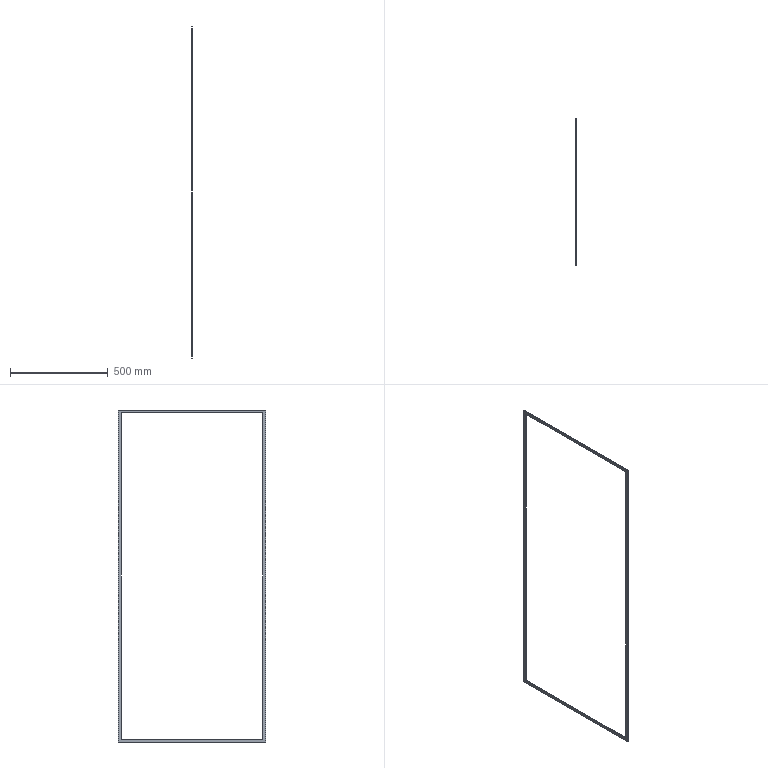Part | STEP file | 1 solid | 10 faces | box 3 x 754 x 1702 mm | volume 218295 mm3 | plane 10
STEP:
#1=CARTESIAN_POINT('',(0.,0.,0.));
#2=DIRECTION('',(0.,0.,1.));
#3=DIRECTION('',(1.,0.,0.));
#4=AXIS2_PLACEMENT_3D('',#1,#2,#3);
#5=CARTESIAN_POINT('',(-521.773,5742.073,1720.144));
#6=VERTEX_POINT('',#5);
#7=CARTESIAN_POINT('',(-521.773,5018.073,1720.144));
#8=VERTEX_POINT('',#7);
#9=CARTESIAN_POINT('',(-521.773,5742.073,1720.144));
#10=DIRECTION('',(0.,-1.,0.));
#11=VECTOR('',#10,1.);
#12=LINE('',#9,#11);
#13=CARTESIAN_POINT('',(-524.773,5003.073,1720.144));
#14=DIRECTION('',(0.,0.,-1.));
#15=DIRECTION('',(0.,-1.,0.));
#16=AXIS2_PLACEMENT_3D('',#13,#14,#15);
#17=PLANE('',#16);
#18=CARTESIAN_POINT('',(-739.,-3.));
#19=DIRECTION('',(1.,0.));
#20=VECTOR('',#19,1.);
#21=LINE('',#18,#20);
#22=(GEOMETRIC_REPRESENTATION_CONTEXT(2)PARAMETRIC_REPRESENTATION_CONTEXT()REPRESENTATION_CONTEXT('',''));
#23=DEFINITIONAL_REPRESENTATION('',(#21),#22);
#24=PCURVE('',#17,#23);
#25=CARTESIAN_POINT('',(-521.773,5003.073,884.394));
#26=DIRECTION('',(1.,0.,0.));
#27=DIRECTION('',(0.,0.,1.));
#28=AXIS2_PLACEMENT_3D('',#25,#26,#27);
#29=PLANE('',#28);
#30=CARTESIAN_POINT('',(835.75,-739.));
#31=DIRECTION('',(0.,1.));
#32=VECTOR('',#31,1.);
#33=LINE('',#30,#32);
#34=(GEOMETRIC_REPRESENTATION_CONTEXT(2)PARAMETRIC_REPRESENTATION_CONTEXT()REPRESENTATION_CONTEXT('',''));
#35=DEFINITIONAL_REPRESENTATION('',(#33),#34);
#36=PCURVE('',#29,#35);
#37=SURFACE_CURVE('',#12,(#24,#36),.PCURVE_S1.);
#38=EDGE_CURVE('',#6,#8,#37,.T.);
#39=ORIENTED_EDGE('',*,*,#38,.F.);
#40=CARTESIAN_POINT('',(-524.773,5742.073,1720.144));
#41=VERTEX_POINT('',#40);
#42=CARTESIAN_POINT('',(-521.773,5742.073,1720.144));
#43=DIRECTION('',(-1.,0.,0.));
#44=VECTOR('',#43,1.);
#45=LINE('',#42,#44);
#46=CARTESIAN_POINT('',(-739.,-3.));
#47=DIRECTION('',(0.,1.));
#48=VECTOR('',#47,1.);
#49=LINE('',#46,#48);
#50=(GEOMETRIC_REPRESENTATION_CONTEXT(2)PARAMETRIC_REPRESENTATION_CONTEXT()REPRESENTATION_CONTEXT('',''));
#51=DEFINITIONAL_REPRESENTATION('',(#49),#50);
#52=PCURVE('',#17,#51);
#53=CARTESIAN_POINT('',(-524.773,5742.073,1720.144));
#54=DIRECTION('',(0.,-1.,0.));
#55=DIRECTION('',(0.,0.,1.));
#56=AXIS2_PLACEMENT_3D('',#53,#54,#55);
#57=PLANE('',#56);
#58=CARTESIAN_POINT('',(0.,-3.));
#59=DIRECTION('',(0.,1.));
#60=VECTOR('',#59,1.);
#61=LINE('',#58,#60);
#62=(GEOMETRIC_REPRESENTATION_CONTEXT(2)PARAMETRIC_REPRESENTATION_CONTEXT()REPRESENTATION_CONTEXT('',''));
#63=DEFINITIONAL_REPRESENTATION('',(#61),#62);
#64=PCURVE('',#57,#63);
#65=SURFACE_CURVE('',#45,(#52,#64),.PCURVE_S1.);
#66=EDGE_CURVE('',#6,#41,#65,.T.);
#67=ORIENTED_EDGE('',*,*,#66,.T.);
#68=CARTESIAN_POINT('',(-524.773,5018.073,1720.144));
#69=VERTEX_POINT('',#68);
#70=CARTESIAN_POINT('',(-524.773,5742.073,1720.144));
#71=DIRECTION('',(0.,-1.,0.));
#72=VECTOR('',#71,1.);
#73=LINE('',#70,#72);
#74=CARTESIAN_POINT('',(-739.,0.));
#75=DIRECTION('',(1.,0.));
#76=VECTOR('',#75,1.);
#77=LINE('',#74,#76);
#78=(GEOMETRIC_REPRESENTATION_CONTEXT(2)PARAMETRIC_REPRESENTATION_CONTEXT()REPRESENTATION_CONTEXT('',''));
#79=DEFINITIONAL_REPRESENTATION('',(#77),#78);
#80=PCURVE('',#17,#79);
#81=CARTESIAN_POINT('',(-524.773,5003.073,884.394));
#82=DIRECTION('',(1.,0.,0.));
#83=DIRECTION('',(0.,0.,1.));
#84=AXIS2_PLACEMENT_3D('',#81,#82,#83);
#85=PLANE('',#84);
#86=CARTESIAN_POINT('',(835.75,-739.));
#87=DIRECTION('',(0.,1.));
#88=VECTOR('',#87,1.);
#89=LINE('',#86,#88);
#90=(GEOMETRIC_REPRESENTATION_CONTEXT(2)PARAMETRIC_REPRESENTATION_CONTEXT()REPRESENTATION_CONTEXT('',''));
#91=DEFINITIONAL_REPRESENTATION('',(#89),#90);
#92=PCURVE('',#85,#91);
#93=SURFACE_CURVE('',#73,(#80,#92),.PCURVE_S1.);
#94=EDGE_CURVE('',#41,#69,#93,.T.);
#95=ORIENTED_EDGE('',*,*,#94,.T.);
#96=CARTESIAN_POINT('',(-524.773,5018.073,1720.144));
#97=DIRECTION('',(1.,0.,0.));
#98=VECTOR('',#97,1.);
#99=LINE('',#96,#98);
#100=CARTESIAN_POINT('',(-15.,0.));
#101=DIRECTION('',(0.,-1.));
#102=VECTOR('',#101,1.);
#103=LINE('',#100,#102);
#104=(GEOMETRIC_REPRESENTATION_CONTEXT(2)PARAMETRIC_REPRESENTATION_CONTEXT()REPRESENTATION_CONTEXT('',''));
#105=DEFINITIONAL_REPRESENTATION('',(#103),#104);
#106=PCURVE('',#17,#105);
#107=CARTESIAN_POINT('',(-521.773,5018.073,1720.144));
#108=DIRECTION('',(0.,1.,0.));
#109=DIRECTION('',(0.,0.,1.));
#110=AXIS2_PLACEMENT_3D('',#107,#108,#109);
#111=PLANE('',#110);
#112=CARTESIAN_POINT('',(0.,-3.));
#113=DIRECTION('',(0.,1.));
#114=VECTOR('',#113,1.);
#115=LINE('',#112,#114);
#116=(GEOMETRIC_REPRESENTATION_CONTEXT(2)PARAMETRIC_REPRESENTATION_CONTEXT()REPRESENTATION_CONTEXT('',''));
#117=DEFINITIONAL_REPRESENTATION('',(#115),#116);
#118=PCURVE('',#111,#117);
#119=SURFACE_CURVE('',#99,(#106,#118),.PCURVE_S1.);
#120=EDGE_CURVE('',#69,#8,#119,.T.);
#121=ORIENTED_EDGE('',*,*,#120,.T.);
#122=EDGE_LOOP('',(#39,#67,#95,#121));
#123=FACE_BOUND('',#122,.F.);
#124=ADVANCED_FACE('',(#123),#17,.T.);
#125=CARTESIAN_POINT('',(-521.773,5003.073,33.644));
#126=VERTEX_POINT('',#125);
#127=CARTESIAN_POINT('',(-521.773,5003.073,1735.144));
#128=VERTEX_POINT('',#127);
#129=CARTESIAN_POINT('',(-521.773,5003.073,33.644));
#130=DIRECTION('',(0.,0.,1.));
#131=VECTOR('',#130,1.);
#132=LINE('',#129,#131);
#133=CARTESIAN_POINT('',(-850.75,0.));
#134=DIRECTION('',(1.,0.));
#135=VECTOR('',#134,1.);
#136=LINE('',#133,#135);
#137=(GEOMETRIC_REPRESENTATION_CONTEXT(2)PARAMETRIC_REPRESENTATION_CONTEXT()REPRESENTATION_CONTEXT('',''));
#138=DEFINITIONAL_REPRESENTATION('',(#136),#137);
#139=PCURVE('',#29,#138);
#140=CARTESIAN_POINT('',(-524.773,5003.073,1735.144));
#141=DIRECTION('',(0.,-1.,0.));
#142=DIRECTION('',(0.,0.,1.));
#143=AXIS2_PLACEMENT_3D('',#140,#141,#142);
#144=PLANE('',#143);
#145=CARTESIAN_POINT('',(-1701.5,-3.));
#146=DIRECTION('',(1.,0.));
#147=VECTOR('',#146,1.);
#148=LINE('',#145,#147);
#149=(GEOMETRIC_REPRESENTATION_CONTEXT(2)PARAMETRIC_REPRESENTATION_CONTEXT()REPRESENTATION_CONTEXT('',''));
#150=DEFINITIONAL_REPRESENTATION('',(#148),#149);
#151=PCURVE('',#144,#150);
#152=SURFACE_CURVE('',#132,(#139,#151),.PCURVE_S1.);
#153=EDGE_CURVE('',#126,#128,#152,.T.);
#154=ORIENTED_EDGE('',*,*,#153,.T.);
#155=CARTESIAN_POINT('',(-521.773,5757.073,1735.144));
#156=VERTEX_POINT('',#155);
#157=CARTESIAN_POINT('',(-521.773,5003.073,1735.144));
#158=DIRECTION('',(0.,1.,0.));
#159=VECTOR('',#158,1.);
#160=LINE('',#157,#159);
#161=CARTESIAN_POINT('',(850.75,0.));
#162=DIRECTION('',(0.,-1.));
#163=VECTOR('',#162,1.);
#164=LINE('',#161,#163);
#165=(GEOMETRIC_REPRESENTATION_CONTEXT(2)PARAMETRIC_REPRESENTATION_CONTEXT()REPRESENTATION_CONTEXT('',''));
#166=DEFINITIONAL_REPRESENTATION('',(#164),#165);
#167=PCURVE('',#29,#166);
#168=CARTESIAN_POINT('',(-524.773,5757.073,1735.144));
#169=DIRECTION('',(0.,0.,1.));
#170=DIRECTION('',(0.,1.,0.));
#171=AXIS2_PLACEMENT_3D('',#168,#169,#170);
#172=PLANE('',#171);
#173=CARTESIAN_POINT('',(-754.,-3.));
#174=DIRECTION('',(1.,0.));
#175=VECTOR('',#174,1.);
#176=LINE('',#173,#175);
#177=(GEOMETRIC_REPRESENTATION_CONTEXT(2)PARAMETRIC_REPRESENTATION_CONTEXT()REPRESENTATION_CONTEXT('',''));
#178=DEFINITIONAL_REPRESENTATION('',(#176),#177);
#179=PCURVE('',#172,#178);
#180=SURFACE_CURVE('',#160,(#167,#179),.PCURVE_S1.);
#181=EDGE_CURVE('',#128,#156,#180,.T.);
#182=ORIENTED_EDGE('',*,*,#181,.T.);
#183=CARTESIAN_POINT('',(-521.773,5757.073,33.644));
#184=VERTEX_POINT('',#183);
#185=CARTESIAN_POINT('',(-521.773,5757.073,1735.144));
#186=DIRECTION('',(0.,0.,-1.));
#187=VECTOR('',#186,1.);
#188=LINE('',#185,#187);
#189=CARTESIAN_POINT('',(850.75,-754.));
#190=DIRECTION('',(-1.,0.));
#191=VECTOR('',#190,1.);
#192=LINE('',#189,#191);
#193=(GEOMETRIC_REPRESENTATION_CONTEXT(2)PARAMETRIC_REPRESENTATION_CONTEXT()REPRESENTATION_CONTEXT('',''));
#194=DEFINITIONAL_REPRESENTATION('',(#192),#193);
#195=PCURVE('',#29,#194);
#196=CARTESIAN_POINT('',(-524.773,5757.073,33.644));
#197=DIRECTION('',(0.,1.,0.));
#198=DIRECTION('',(0.,0.,-1.));
#199=AXIS2_PLACEMENT_3D('',#196,#197,#198);
#200=PLANE('',#199);
#201=CARTESIAN_POINT('',(-1701.5,-3.));
#202=DIRECTION('',(1.,0.));
#203=VECTOR('',#202,1.);
#204=LINE('',#201,#203);
#205=(GEOMETRIC_REPRESENTATION_CONTEXT(2)PARAMETRIC_REPRESENTATION_CONTEXT()REPRESENTATION_CONTEXT('',''));
#206=DEFINITIONAL_REPRESENTATION('',(#204),#205);
#207=PCURVE('',#200,#206);
#208=SURFACE_CURVE('',#188,(#195,#207),.PCURVE_S1.);
#209=EDGE_CURVE('',#156,#184,#208,.T.);
#210=ORIENTED_EDGE('',*,*,#209,.T.);
#211=CARTESIAN_POINT('',(-521.773,5757.073,33.644));
#212=DIRECTION('',(0.,-1.,0.));
#213=VECTOR('',#212,1.);
#214=LINE('',#211,#213);
#215=CARTESIAN_POINT('',(-850.75,-754.));
#216=DIRECTION('',(0.,1.));
#217=VECTOR('',#216,1.);
#218=LINE('',#215,#217);
#219=(GEOMETRIC_REPRESENTATION_CONTEXT(2)PARAMETRIC_REPRESENTATION_CONTEXT()REPRESENTATION_CONTEXT('',''));
#220=DEFINITIONAL_REPRESENTATION('',(#218),#219);
#221=PCURVE('',#29,#220);
#222=CARTESIAN_POINT('',(-524.773,5003.073,33.644));
#223=DIRECTION('',(0.,0.,-1.));
#224=DIRECTION('',(0.,-1.,0.));
#225=AXIS2_PLACEMENT_3D('',#222,#223,#224);
#226=PLANE('',#225);
#227=CARTESIAN_POINT('',(-754.,-3.));
#228=DIRECTION('',(1.,0.));
#229=VECTOR('',#228,1.);
#230=LINE('',#227,#229);
#231=(GEOMETRIC_REPRESENTATION_CONTEXT(2)PARAMETRIC_REPRESENTATION_CONTEXT()REPRESENTATION_CONTEXT('',''));
#232=DEFINITIONAL_REPRESENTATION('',(#230),#231);
#233=PCURVE('',#226,#232);
#234=SURFACE_CURVE('',#214,(#221,#233),.PCURVE_S1.);
#235=EDGE_CURVE('',#184,#126,#234,.T.);
#236=ORIENTED_EDGE('',*,*,#235,.T.);
#237=EDGE_LOOP('',(#154,#182,#210,#236));
#238=FACE_BOUND('',#237,.F.);
#239=CARTESIAN_POINT('',(-521.773,5018.073,48.644));
#240=VERTEX_POINT('',#239);
#241=CARTESIAN_POINT('',(-521.773,5018.073,48.644));
#242=DIRECTION('',(0.,0.,1.));
#243=VECTOR('',#242,1.);
#244=LINE('',#241,#243);
#245=CARTESIAN_POINT('',(-835.75,-15.));
#246=DIRECTION('',(1.,0.));
#247=VECTOR('',#246,1.);
#248=LINE('',#245,#247);
#249=(GEOMETRIC_REPRESENTATION_CONTEXT(2)PARAMETRIC_REPRESENTATION_CONTEXT()REPRESENTATION_CONTEXT('',''));
#250=DEFINITIONAL_REPRESENTATION('',(#248),#249);
#251=PCURVE('',#29,#250);
#252=CARTESIAN_POINT('',(-1671.5,0.));
#253=DIRECTION('',(1.,0.));
#254=VECTOR('',#253,1.);
#255=LINE('',#252,#254);
#256=(GEOMETRIC_REPRESENTATION_CONTEXT(2)PARAMETRIC_REPRESENTATION_CONTEXT()REPRESENTATION_CONTEXT('',''));
#257=DEFINITIONAL_REPRESENTATION('',(#255),#256);
#258=PCURVE('',#111,#257);
#259=SURFACE_CURVE('',#244,(#251,#258),.PCURVE_S1.);
#260=EDGE_CURVE('',#240,#8,#259,.T.);
#261=ORIENTED_EDGE('',*,*,#260,.F.);
#262=CARTESIAN_POINT('',(-521.773,5742.073,48.644));
#263=VERTEX_POINT('',#262);
#264=CARTESIAN_POINT('',(-521.773,5018.073,48.644));
#265=DIRECTION('',(0.,1.,0.));
#266=VECTOR('',#265,1.);
#267=LINE('',#264,#266);
#268=CARTESIAN_POINT('',(-835.75,-15.));
#269=DIRECTION('',(0.,-1.));
#270=VECTOR('',#269,1.);
#271=LINE('',#268,#270);
#272=(GEOMETRIC_REPRESENTATION_CONTEXT(2)PARAMETRIC_REPRESENTATION_CONTEXT()REPRESENTATION_CONTEXT('',''));
#273=DEFINITIONAL_REPRESENTATION('',(#271),#272);
#274=PCURVE('',#29,#273);
#275=CARTESIAN_POINT('',(-524.773,5742.073,48.644));
#276=DIRECTION('',(0.,0.,1.));
#277=DIRECTION('',(0.,1.,0.));
#278=AXIS2_PLACEMENT_3D('',#275,#276,#277);
#279=PLANE('',#278);
#280=CARTESIAN_POINT('',(-724.,-3.));
#281=DIRECTION('',(1.,0.));
#282=VECTOR('',#281,1.);
#283=LINE('',#280,#282);
#284=(GEOMETRIC_REPRESENTATION_CONTEXT(2)PARAMETRIC_REPRESENTATION_CONTEXT()REPRESENTATION_CONTEXT('',''));
#285=DEFINITIONAL_REPRESENTATION('',(#283),#284);
#286=PCURVE('',#279,#285);
#287=SURFACE_CURVE('',#267,(#274,#286),.PCURVE_S1.);
#288=EDGE_CURVE('',#240,#263,#287,.T.);
#289=ORIENTED_EDGE('',*,*,#288,.T.);
#290=CARTESIAN_POINT('',(-521.773,5742.073,48.644));
#291=DIRECTION('',(0.,0.,1.));
#292=VECTOR('',#291,1.);
#293=LINE('',#290,#292);
#294=CARTESIAN_POINT('',(-835.75,-739.));
#295=DIRECTION('',(1.,0.));
#296=VECTOR('',#295,1.);
#297=LINE('',#294,#296);
#298=(GEOMETRIC_REPRESENTATION_CONTEXT(2)PARAMETRIC_REPRESENTATION_CONTEXT()REPRESENTATION_CONTEXT('',''));
#299=DEFINITIONAL_REPRESENTATION('',(#297),#298);
#300=PCURVE('',#29,#299);
#301=CARTESIAN_POINT('',(-1671.5,-3.));
#302=DIRECTION('',(1.,0.));
#303=VECTOR('',#302,1.);
#304=LINE('',#301,#303);
#305=(GEOMETRIC_REPRESENTATION_CONTEXT(2)PARAMETRIC_REPRESENTATION_CONTEXT()REPRESENTATION_CONTEXT('',''));
#306=DEFINITIONAL_REPRESENTATION('',(#304),#305);
#307=PCURVE('',#57,#306);
#308=SURFACE_CURVE('',#293,(#300,#307),.PCURVE_S1.);
#309=EDGE_CURVE('',#263,#6,#308,.T.);
#310=ORIENTED_EDGE('',*,*,#309,.T.);
#311=ORIENTED_EDGE('',*,*,#38,.T.);
#312=EDGE_LOOP('',(#261,#289,#310,#311));
#313=FACE_BOUND('',#312,.F.);
#314=ADVANCED_FACE('',(#238,#313),#29,.T.);
#315=CARTESIAN_POINT('',(-524.773,5018.073,48.644));
#316=VERTEX_POINT('',#315);
#317=CARTESIAN_POINT('',(-524.773,5018.073,48.644));
#318=DIRECTION('',(0.,0.,1.));
#319=VECTOR('',#318,1.);
#320=LINE('',#317,#319);
#321=CARTESIAN_POINT('',(-1671.5,-3.));
#322=DIRECTION('',(1.,0.));
#323=VECTOR('',#322,1.);
#324=LINE('',#321,#323);
#325=(GEOMETRIC_REPRESENTATION_CONTEXT(2)PARAMETRIC_REPRESENTATION_CONTEXT()REPRESENTATION_CONTEXT('',''));
#326=DEFINITIONAL_REPRESENTATION('',(#324),#325);
#327=PCURVE('',#111,#326);
#328=CARTESIAN_POINT('',(-835.75,-15.));
#329=DIRECTION('',(1.,0.));
#330=VECTOR('',#329,1.);
#331=LINE('',#328,#330);
#332=(GEOMETRIC_REPRESENTATION_CONTEXT(2)PARAMETRIC_REPRESENTATION_CONTEXT()REPRESENTATION_CONTEXT('',''));
#333=DEFINITIONAL_REPRESENTATION('',(#331),#332);
#334=PCURVE('',#85,#333);
#335=SURFACE_CURVE('',#320,(#327,#334),.PCURVE_S1.);
#336=EDGE_CURVE('',#316,#69,#335,.T.);
#337=ORIENTED_EDGE('',*,*,#336,.F.);
#338=CARTESIAN_POINT('',(-524.773,5018.073,48.644));
#339=DIRECTION('',(1.,0.,0.));
#340=VECTOR('',#339,1.);
#341=LINE('',#338,#340);
#342=CARTESIAN_POINT('',(-1671.5,-3.));
#343=DIRECTION('',(0.,1.));
#344=VECTOR('',#343,1.);
#345=LINE('',#342,#344);
#346=(GEOMETRIC_REPRESENTATION_CONTEXT(2)PARAMETRIC_REPRESENTATION_CONTEXT()REPRESENTATION_CONTEXT('',''));
#347=DEFINITIONAL_REPRESENTATION('',(#345),#346);
#348=PCURVE('',#111,#347);
#349=CARTESIAN_POINT('',(-724.,0.));
#350=DIRECTION('',(0.,-1.));
#351=VECTOR('',#350,1.);
#352=LINE('',#349,#351);
#353=(GEOMETRIC_REPRESENTATION_CONTEXT(2)PARAMETRIC_REPRESENTATION_CONTEXT()REPRESENTATION_CONTEXT('',''));
#354=DEFINITIONAL_REPRESENTATION('',(#352),#353);
#355=PCURVE('',#279,#354);
#356=SURFACE_CURVE('',#341,(#348,#355),.PCURVE_S1.);
#357=EDGE_CURVE('',#316,#240,#356,.T.);
#358=ORIENTED_EDGE('',*,*,#357,.T.);
#359=ORIENTED_EDGE('',*,*,#260,.T.);
#360=ORIENTED_EDGE('',*,*,#120,.F.);
#361=EDGE_LOOP('',(#337,#358,#359,#360));
#362=FACE_BOUND('',#361,.F.);
#363=ADVANCED_FACE('',(#362),#111,.T.);
#364=CARTESIAN_POINT('',(-524.773,5003.073,33.644));
#365=VERTEX_POINT('',#364);
#366=CARTESIAN_POINT('',(-524.773,5003.073,1735.144));
#367=VERTEX_POINT('',#366);
#368=CARTESIAN_POINT('',(-524.773,5003.073,33.644));
#369=DIRECTION('',(0.,0.,1.));
#370=VECTOR('',#369,1.);
#371=LINE('',#368,#370);
#372=CARTESIAN_POINT('',(-850.75,0.));
#373=DIRECTION('',(1.,0.));
#374=VECTOR('',#373,1.);
#375=LINE('',#372,#374);
#376=(GEOMETRIC_REPRESENTATION_CONTEXT(2)PARAMETRIC_REPRESENTATION_CONTEXT()REPRESENTATION_CONTEXT('',''));
#377=DEFINITIONAL_REPRESENTATION('',(#375),#376);
#378=PCURVE('',#85,#377);
#379=CARTESIAN_POINT('',(-1701.5,0.));
#380=DIRECTION('',(1.,0.));
#381=VECTOR('',#380,1.);
#382=LINE('',#379,#381);
#383=(GEOMETRIC_REPRESENTATION_CONTEXT(2)PARAMETRIC_REPRESENTATION_CONTEXT()REPRESENTATION_CONTEXT('',''));
#384=DEFINITIONAL_REPRESENTATION('',(#382),#383);
#385=PCURVE('',#144,#384);
#386=SURFACE_CURVE('',#371,(#378,#385),.PCURVE_S1.);
#387=EDGE_CURVE('',#365,#367,#386,.T.);
#388=ORIENTED_EDGE('',*,*,#387,.F.);
#389=CARTESIAN_POINT('',(-524.773,5757.073,33.644));
#390=VERTEX_POINT('',#389);
#391=CARTESIAN_POINT('',(-524.773,5757.073,33.644));
#392=DIRECTION('',(0.,-1.,0.));
#393=VECTOR('',#392,1.);
#394=LINE('',#391,#393);
#395=CARTESIAN_POINT('',(-850.75,-754.));
#396=DIRECTION('',(0.,1.));
#397=VECTOR('',#396,1.);
#398=LINE('',#395,#397);
#399=(GEOMETRIC_REPRESENTATION_CONTEXT(2)PARAMETRIC_REPRESENTATION_CONTEXT()REPRESENTATION_CONTEXT('',''));
#400=DEFINITIONAL_REPRESENTATION('',(#398),#399);
#401=PCURVE('',#85,#400);
#402=CARTESIAN_POINT('',(-754.,0.));
#403=DIRECTION('',(1.,0.));
#404=VECTOR('',#403,1.);
#405=LINE('',#402,#404);
#406=(GEOMETRIC_REPRESENTATION_CONTEXT(2)PARAMETRIC_REPRESENTATION_CONTEXT()REPRESENTATION_CONTEXT('',''));
#407=DEFINITIONAL_REPRESENTATION('',(#405),#406);
#408=PCURVE('',#226,#407);
#409=SURFACE_CURVE('',#394,(#401,#408),.PCURVE_S1.);
#410=EDGE_CURVE('',#390,#365,#409,.T.);
#411=ORIENTED_EDGE('',*,*,#410,.F.);
#412=CARTESIAN_POINT('',(-524.773,5757.073,1735.144));
#413=VERTEX_POINT('',#412);
#414=CARTESIAN_POINT('',(-524.773,5757.073,1735.144));
#415=DIRECTION('',(0.,0.,-1.));
#416=VECTOR('',#415,1.);
#417=LINE('',#414,#416);
#418=CARTESIAN_POINT('',(850.75,-754.));
#419=DIRECTION('',(-1.,0.));
#420=VECTOR('',#419,1.);
#421=LINE('',#418,#420);
#422=(GEOMETRIC_REPRESENTATION_CONTEXT(2)PARAMETRIC_REPRESENTATION_CONTEXT()REPRESENTATION_CONTEXT('',''));
#423=DEFINITIONAL_REPRESENTATION('',(#421),#422);
#424=PCURVE('',#85,#423);
#425=CARTESIAN_POINT('',(-1701.5,0.));
#426=DIRECTION('',(1.,0.));
#427=VECTOR('',#426,1.);
#428=LINE('',#425,#427);
#429=(GEOMETRIC_REPRESENTATION_CONTEXT(2)PARAMETRIC_REPRESENTATION_CONTEXT()REPRESENTATION_CONTEXT('',''));
#430=DEFINITIONAL_REPRESENTATION('',(#428),#429);
#431=PCURVE('',#200,#430);
#432=SURFACE_CURVE('',#417,(#424,#431),.PCURVE_S1.);
#433=EDGE_CURVE('',#413,#390,#432,.T.);
#434=ORIENTED_EDGE('',*,*,#433,.F.);
#435=CARTESIAN_POINT('',(-524.773,5003.073,1735.144));
#436=DIRECTION('',(0.,1.,0.));
#437=VECTOR('',#436,1.);
#438=LINE('',#435,#437);
#439=CARTESIAN_POINT('',(850.75,0.));
#440=DIRECTION('',(0.,-1.));
#441=VECTOR('',#440,1.);
#442=LINE('',#439,#441);
#443=(GEOMETRIC_REPRESENTATION_CONTEXT(2)PARAMETRIC_REPRESENTATION_CONTEXT()REPRESENTATION_CONTEXT('',''));
#444=DEFINITIONAL_REPRESENTATION('',(#442),#443);
#445=PCURVE('',#85,#444);
#446=CARTESIAN_POINT('',(-754.,0.));
#447=DIRECTION('',(1.,0.));
#448=VECTOR('',#447,1.);
#449=LINE('',#446,#448);
#450=(GEOMETRIC_REPRESENTATION_CONTEXT(2)PARAMETRIC_REPRESENTATION_CONTEXT()REPRESENTATION_CONTEXT('',''));
#451=DEFINITIONAL_REPRESENTATION('',(#449),#450);
#452=PCURVE('',#172,#451);
#453=SURFACE_CURVE('',#438,(#445,#452),.PCURVE_S1.);
#454=EDGE_CURVE('',#367,#413,#453,.T.);
#455=ORIENTED_EDGE('',*,*,#454,.F.);
#456=EDGE_LOOP('',(#388,#411,#434,#455));
#457=FACE_BOUND('',#456,.F.);
#458=ORIENTED_EDGE('',*,*,#94,.F.);
#459=CARTESIAN_POINT('',(-524.773,5742.073,48.644));
#460=VERTEX_POINT('',#459);
#461=CARTESIAN_POINT('',(-524.773,5742.073,48.644));
#462=DIRECTION('',(0.,0.,1.));
#463=VECTOR('',#462,1.);
#464=LINE('',#461,#463);
#465=CARTESIAN_POINT('',(-835.75,-739.));
#466=DIRECTION('',(1.,0.));
#467=VECTOR('',#466,1.);
#468=LINE('',#465,#467);
#469=(GEOMETRIC_REPRESENTATION_CONTEXT(2)PARAMETRIC_REPRESENTATION_CONTEXT()REPRESENTATION_CONTEXT('',''));
#470=DEFINITIONAL_REPRESENTATION('',(#468),#469);
#471=PCURVE('',#85,#470);
#472=CARTESIAN_POINT('',(-1671.5,0.));
#473=DIRECTION('',(1.,0.));
#474=VECTOR('',#473,1.);
#475=LINE('',#472,#474);
#476=(GEOMETRIC_REPRESENTATION_CONTEXT(2)PARAMETRIC_REPRESENTATION_CONTEXT()REPRESENTATION_CONTEXT('',''));
#477=DEFINITIONAL_REPRESENTATION('',(#475),#476);
#478=PCURVE('',#57,#477);
#479=SURFACE_CURVE('',#464,(#471,#478),.PCURVE_S1.);
#480=EDGE_CURVE('',#460,#41,#479,.T.);
#481=ORIENTED_EDGE('',*,*,#480,.F.);
#482=CARTESIAN_POINT('',(-524.773,5018.073,48.644));
#483=DIRECTION('',(0.,1.,0.));
#484=VECTOR('',#483,1.);
#485=LINE('',#482,#484);
#486=CARTESIAN_POINT('',(-835.75,-15.));
#487=DIRECTION('',(0.,-1.));
#488=VECTOR('',#487,1.);
#489=LINE('',#486,#488);
#490=(GEOMETRIC_REPRESENTATION_CONTEXT(2)PARAMETRIC_REPRESENTATION_CONTEXT()REPRESENTATION_CONTEXT('',''));
#491=DEFINITIONAL_REPRESENTATION('',(#489),#490);
#492=PCURVE('',#85,#491);
#493=CARTESIAN_POINT('',(-724.,0.));
#494=DIRECTION('',(1.,0.));
#495=VECTOR('',#494,1.);
#496=LINE('',#493,#495);
#497=(GEOMETRIC_REPRESENTATION_CONTEXT(2)PARAMETRIC_REPRESENTATION_CONTEXT()REPRESENTATION_CONTEXT('',''));
#498=DEFINITIONAL_REPRESENTATION('',(#496),#497);
#499=PCURVE('',#279,#498);
#500=SURFACE_CURVE('',#485,(#492,#499),.PCURVE_S1.);
#501=EDGE_CURVE('',#316,#460,#500,.T.);
#502=ORIENTED_EDGE('',*,*,#501,.F.);
#503=ORIENTED_EDGE('',*,*,#336,.T.);
#504=EDGE_LOOP('',(#458,#481,#502,#503));
#505=FACE_BOUND('',#504,.F.);
#506=ADVANCED_FACE('',(#457,#505),#85,.F.);
#507=CARTESIAN_POINT('',(-521.773,5742.073,48.644));
#508=DIRECTION('',(-1.,0.,0.));
#509=VECTOR('',#508,1.);
#510=LINE('',#507,#509);
#511=CARTESIAN_POINT('',(-1671.5,-3.));
#512=DIRECTION('',(0.,1.));
#513=VECTOR('',#512,1.);
#514=LINE('',#511,#513);
#515=(GEOMETRIC_REPRESENTATION_CONTEXT(2)PARAMETRIC_REPRESENTATION_CONTEXT()REPRESENTATION_CONTEXT('',''));
#516=DEFINITIONAL_REPRESENTATION('',(#514),#515);
#517=PCURVE('',#57,#516);
#518=CARTESIAN_POINT('',(0.,-3.));
#519=DIRECTION('',(0.,1.));
#520=VECTOR('',#519,1.);
#521=LINE('',#518,#520);
#522=(GEOMETRIC_REPRESENTATION_CONTEXT(2)PARAMETRIC_REPRESENTATION_CONTEXT()REPRESENTATION_CONTEXT('',''));
#523=DEFINITIONAL_REPRESENTATION('',(#521),#522);
#524=PCURVE('',#279,#523);
#525=SURFACE_CURVE('',#510,(#517,#524),.PCURVE_S1.);
#526=EDGE_CURVE('',#263,#460,#525,.T.);
#527=ORIENTED_EDGE('',*,*,#526,.T.);
#528=ORIENTED_EDGE('',*,*,#480,.T.);
#529=ORIENTED_EDGE('',*,*,#66,.F.);
#530=ORIENTED_EDGE('',*,*,#309,.F.);
#531=EDGE_LOOP('',(#527,#528,#529,#530));
#532=FACE_BOUND('',#531,.F.);
#533=ADVANCED_FACE('',(#532),#57,.T.);
#534=ORIENTED_EDGE('',*,*,#357,.F.);
#535=ORIENTED_EDGE('',*,*,#501,.T.);
#536=ORIENTED_EDGE('',*,*,#526,.F.);
#537=ORIENTED_EDGE('',*,*,#288,.F.);
#538=EDGE_LOOP('',(#534,#535,#536,#537));
#539=FACE_BOUND('',#538,.F.);
#540=ADVANCED_FACE('',(#539),#279,.T.);
#541=CARTESIAN_POINT('',(-521.773,5003.073,1735.144));
#542=DIRECTION('',(-1.,0.,0.));
#543=VECTOR('',#542,1.);
#544=LINE('',#541,#543);
#545=CARTESIAN_POINT('',(0.,-3.));
#546=DIRECTION('',(0.,1.));
#547=VECTOR('',#546,1.);
#548=LINE('',#545,#547);
#549=(GEOMETRIC_REPRESENTATION_CONTEXT(2)PARAMETRIC_REPRESENTATION_CONTEXT()REPRESENTATION_CONTEXT('',''));
#550=DEFINITIONAL_REPRESENTATION('',(#548),#549);
#551=PCURVE('',#144,#550);
#552=CARTESIAN_POINT('',(-754.,-3.));
#553=DIRECTION('',(0.,1.));
#554=VECTOR('',#553,1.);
#555=LINE('',#552,#554);
#556=(GEOMETRIC_REPRESENTATION_CONTEXT(2)PARAMETRIC_REPRESENTATION_CONTEXT()REPRESENTATION_CONTEXT('',''));
#557=DEFINITIONAL_REPRESENTATION('',(#555),#556);
#558=PCURVE('',#172,#557);
#559=SURFACE_CURVE('',#544,(#551,#558),.PCURVE_S1.);
#560=EDGE_CURVE('',#128,#367,#559,.T.);
#561=ORIENTED_EDGE('',*,*,#560,.F.);
#562=ORIENTED_EDGE('',*,*,#153,.F.);
#563=CARTESIAN_POINT('',(-521.773,5003.073,33.644));
#564=DIRECTION('',(-1.,0.,0.));
#565=VECTOR('',#564,1.);
#566=LINE('',#563,#565);
#567=CARTESIAN_POINT('',(-1701.5,-3.));
#568=DIRECTION('',(0.,1.));
#569=VECTOR('',#568,1.);
#570=LINE('',#567,#569);
#571=(GEOMETRIC_REPRESENTATION_CONTEXT(2)PARAMETRIC_REPRESENTATION_CONTEXT()REPRESENTATION_CONTEXT('',''));
#572=DEFINITIONAL_REPRESENTATION('',(#570),#571);
#573=PCURVE('',#144,#572);
#574=CARTESIAN_POINT('',(0.,-3.));
#575=DIRECTION('',(0.,1.));
#576=VECTOR('',#575,1.);
#577=LINE('',#574,#576);
#578=(GEOMETRIC_REPRESENTATION_CONTEXT(2)PARAMETRIC_REPRESENTATION_CONTEXT()REPRESENTATION_CONTEXT('',''));
#579=DEFINITIONAL_REPRESENTATION('',(#577),#578);
#580=PCURVE('',#226,#579);
#581=SURFACE_CURVE('',#566,(#573,#580),.PCURVE_S1.);
#582=EDGE_CURVE('',#126,#365,#581,.T.);
#583=ORIENTED_EDGE('',*,*,#582,.T.);
#584=ORIENTED_EDGE('',*,*,#387,.T.);
#585=EDGE_LOOP('',(#561,#562,#583,#584));
#586=FACE_BOUND('',#585,.F.);
#587=ADVANCED_FACE('',(#586),#144,.T.);
#588=ORIENTED_EDGE('',*,*,#560,.T.);
#589=ORIENTED_EDGE('',*,*,#454,.T.);
#590=CARTESIAN_POINT('',(-521.773,5757.073,1735.144));
#591=DIRECTION('',(-1.,0.,0.));
#592=VECTOR('',#591,1.);
#593=LINE('',#590,#592);
#594=CARTESIAN_POINT('',(0.,-3.));
#595=DIRECTION('',(0.,1.));
#596=VECTOR('',#595,1.);
#597=LINE('',#594,#596);
#598=(GEOMETRIC_REPRESENTATION_CONTEXT(2)PARAMETRIC_REPRESENTATION_CONTEXT()REPRESENTATION_CONTEXT('',''));
#599=DEFINITIONAL_REPRESENTATION('',(#597),#598);
#600=PCURVE('',#172,#599);
#601=CARTESIAN_POINT('',(-1701.5,-3.));
#602=DIRECTION('',(0.,1.));
#603=VECTOR('',#602,1.);
#604=LINE('',#601,#603);
#605=(GEOMETRIC_REPRESENTATION_CONTEXT(2)PARAMETRIC_REPRESENTATION_CONTEXT()REPRESENTATION_CONTEXT('',''));
#606=DEFINITIONAL_REPRESENTATION('',(#604),#605);
#607=PCURVE('',#200,#606);
#608=SURFACE_CURVE('',#593,(#600,#607),.PCURVE_S1.);
#609=EDGE_CURVE('',#156,#413,#608,.T.);
#610=ORIENTED_EDGE('',*,*,#609,.F.);
#611=ORIENTED_EDGE('',*,*,#181,.F.);
#612=EDGE_LOOP('',(#588,#589,#610,#611));
#613=FACE_BOUND('',#612,.F.);
#614=ADVANCED_FACE('',(#613),#172,.T.);
#615=ORIENTED_EDGE('',*,*,#609,.T.);
#616=ORIENTED_EDGE('',*,*,#433,.T.);
#617=CARTESIAN_POINT('',(-521.773,5757.073,33.644));
#618=DIRECTION('',(-1.,0.,0.));
#619=VECTOR('',#618,1.);
#620=LINE('',#617,#619);
#621=CARTESIAN_POINT('',(0.,-3.));
#622=DIRECTION('',(0.,1.));
#623=VECTOR('',#622,1.);
#624=LINE('',#621,#623);
#625=(GEOMETRIC_REPRESENTATION_CONTEXT(2)PARAMETRIC_REPRESENTATION_CONTEXT()REPRESENTATION_CONTEXT('',''));
#626=DEFINITIONAL_REPRESENTATION('',(#624),#625);
#627=PCURVE('',#200,#626);
#628=CARTESIAN_POINT('',(-754.,-3.));
#629=DIRECTION('',(0.,1.));
#630=VECTOR('',#629,1.);
#631=LINE('',#628,#630);
#632=(GEOMETRIC_REPRESENTATION_CONTEXT(2)PARAMETRIC_REPRESENTATION_CONTEXT()REPRESENTATION_CONTEXT('',''));
#633=DEFINITIONAL_REPRESENTATION('',(#631),#632);
#634=PCURVE('',#226,#633);
#635=SURFACE_CURVE('',#620,(#627,#634),.PCURVE_S1.);
#636=EDGE_CURVE('',#184,#390,#635,.T.);
#637=ORIENTED_EDGE('',*,*,#636,.F.);
#638=ORIENTED_EDGE('',*,*,#209,.F.);
#639=EDGE_LOOP('',(#615,#616,#637,#638));
#640=FACE_BOUND('',#639,.F.);
#641=ADVANCED_FACE('',(#640),#200,.T.);
#642=ORIENTED_EDGE('',*,*,#636,.T.);
#643=ORIENTED_EDGE('',*,*,#410,.T.);
#644=ORIENTED_EDGE('',*,*,#582,.F.);
#645=ORIENTED_EDGE('',*,*,#235,.F.);
#646=EDGE_LOOP('',(#642,#643,#644,#645));
#647=FACE_BOUND('',#646,.F.);
#648=ADVANCED_FACE('',(#647),#226,.T.);
#649=CLOSED_SHELL('',(#124,#314,#363,#506,#533,#540,#587,#614,#641,#648));
#650=MANIFOLD_SOLID_BREP('',#649);
#651=(LENGTH_UNIT()NAMED_UNIT(*)SI_UNIT(.MILLI.,.METRE.));
#652=UNCERTAINTY_MEASURE_WITH_UNIT(LENGTH_MEASURE(0.0000001),#651,'','');
#653=(NAMED_UNIT(*)PLANE_ANGLE_UNIT()SI_UNIT($,.RADIAN.));
#654=(NAMED_UNIT(*)SI_UNIT($,.STERADIAN.)SOLID_ANGLE_UNIT());
#655=(GEOMETRIC_REPRESENTATION_CONTEXT(3)GLOBAL_UNCERTAINTY_ASSIGNED_CONTEXT((#652))GLOBAL_UNIT_ASSIGNED_CONTEXT((#651,#653,#654))REPRESENTATION_CONTEXT('',''));
#656=ADVANCED_BREP_SHAPE_REPRESENTATION('',(#4,#650),#655);